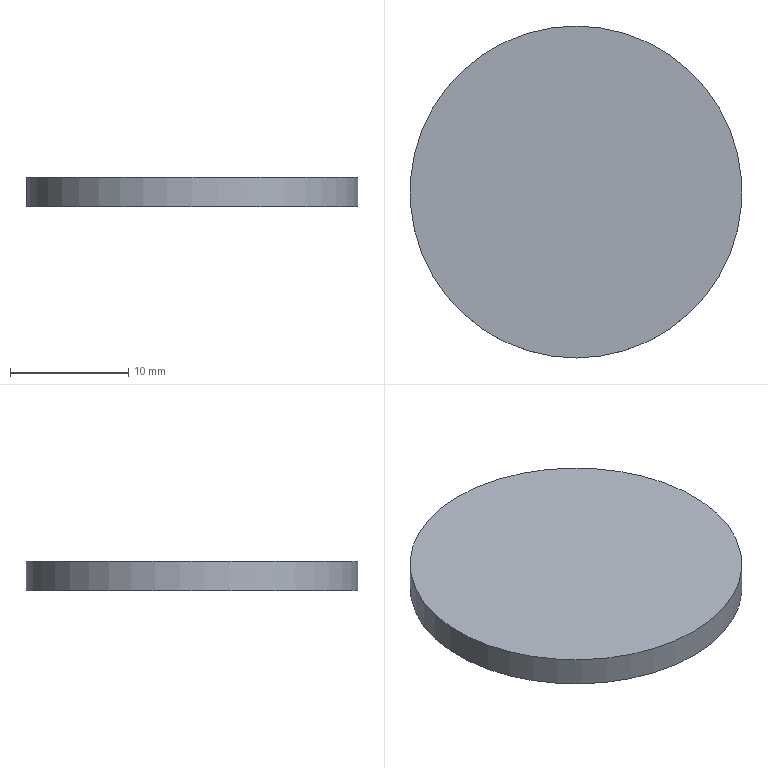Part | STEP file | lll_id1266_x_t | 1 solid | 3 faces | box 28.07 x 28.07 x 2.5 mm | volume 1547 mm3 | plane 2 | cylinder 1 | commonest cylinder face diameters 28.07 x1
STEP:
#1=CARTESIAN_POINT('',(3339.867,-218.323,0.00001711));
#2=VERTEX_POINT('',#1);
#3=CARTESIAN_POINT('',(3339.867,-204.288,0.00001711));
#4=DIRECTION('',(0.000000008,0.,-1.));
#5=DIRECTION('',(0.,-1.,0.));
#6=AXIS2_PLACEMENT_3D('',#3,#4,#5);
#7=CIRCLE('',#6,14.035);
#8=EDGE_CURVE('',#2,#2,#7,.T.);
#9=ORIENTED_EDGE('',*,*,#8,.T.);
#10=EDGE_LOOP('',(#9));
#11=FACE_OUTER_BOUND('',#10,.T.);
#12=CARTESIAN_POINT('',(3339.867,-204.288,0.00001711));
#13=DIRECTION('',(0.000000008,0.,-1.));
#14=DIRECTION('',(0.,-1.,0.));
#15=AXIS2_PLACEMENT_3D('',#12,#13,#14);
#16=PLANE('',#15);
#17=ADVANCED_FACE('',(#11),#16,.T.);
#18=CARTESIAN_POINT('',(3339.867,-218.323,2.5));
#19=VERTEX_POINT('',#18);
#20=CARTESIAN_POINT('',(3339.867,-204.288,2.5));
#21=DIRECTION('',(0.000000008,0.,-1.));
#22=DIRECTION('',(0.,-1.,0.));
#23=AXIS2_PLACEMENT_3D('',#20,#21,#22);
#24=CIRCLE('',#23,14.035);
#25=EDGE_CURVE('',#19,#19,#24,.T.);
#26=ORIENTED_EDGE('',*,*,#25,.F.);
#27=EDGE_LOOP('',(#26));
#28=FACE_OUTER_BOUND('',#27,.T.);
#29=CARTESIAN_POINT('',(3339.867,-204.288,2.5));
#30=DIRECTION('',(-0.000000008,0.,1.));
#31=DIRECTION('',(0.,1.,0.));
#32=AXIS2_PLACEMENT_3D('',#29,#30,#31);
#33=PLANE('',#32);
#34=ADVANCED_FACE('',(#28),#33,.T.);
#35=ORIENTED_EDGE('',*,*,#8,.F.);
#36=EDGE_LOOP('',(#35));
#37=FACE_BOUND('',#36,.T.);
#38=ORIENTED_EDGE('',*,*,#25,.T.);
#39=EDGE_LOOP('',(#38));
#40=FACE_BOUND('',#39,.T.);
#41=CARTESIAN_POINT('',(3339.867,-204.288,2.5));
#42=DIRECTION('',(0.000000008,0.,-1.));
#43=DIRECTION('',(0.,-1.,0.));
#44=AXIS2_PLACEMENT_3D('',#41,#42,#43);
#45=CYLINDRICAL_SURFACE('',#44,14.035);
#46=ADVANCED_FACE('',(#37,#40),#45,.T.);
#47=CLOSED_SHELL('',(#17,#34,#46));
#48=MANIFOLD_SOLID_BREP('',#47);
#49=(LENGTH_UNIT()NAMED_UNIT(*)SI_UNIT(.MILLI.,.METRE.));
#50=UNCERTAINTY_MEASURE_WITH_UNIT(LENGTH_MEASURE(0.00002),#49,'','');
#51=(NAMED_UNIT(*)PLANE_ANGLE_UNIT()SI_UNIT($,.RADIAN.));
#52=PLANE_ANGLE_MEASURE_WITH_UNIT(PLANE_ANGLE_MEASURE(0.01745),#51);
#53=DIMENSIONAL_EXPONENTS(0.,0.,0.,0.,0.,0.,0.);
#54=(CONVERSION_BASED_UNIT('DEGREE',#52)NAMED_UNIT(#53)PLANE_ANGLE_UNIT());
#55=(NAMED_UNIT(*)SI_UNIT($,.STERADIAN.)SOLID_ANGLE_UNIT());
#56=(GEOMETRIC_REPRESENTATION_CONTEXT(3)GLOBAL_UNCERTAINTY_ASSIGNED_CONTEXT((#50))GLOBAL_UNIT_ASSIGNED_CONTEXT((#49,#54,#55))REPRESENTATION_CONTEXT('',''));
#57=ADVANCED_BREP_SHAPE_REPRESENTATION('',(#48),#56);